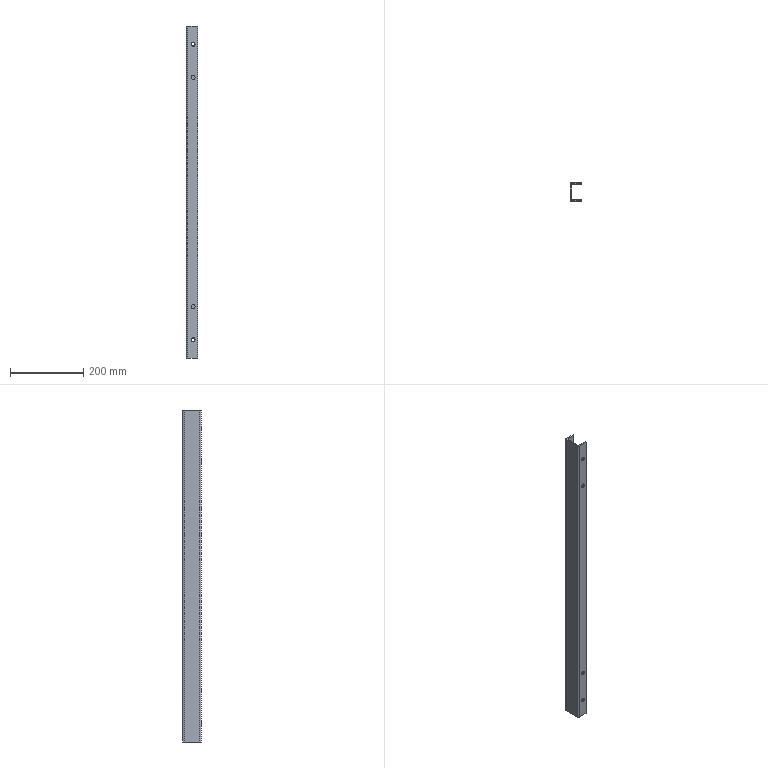Part | SolidWorks | features Cut 1, FlatPattern 1, ICE 1, SMBaseFlange 1, SheetMetal 1 | 1 solid | 55 faces | box 30 x 50 x 905 mm | volume 273080 mm3 | plane 28 | cylinder 27 | commonest cylinder face diameters 10 x15 11 x8 0.4 x2 6.4 x2